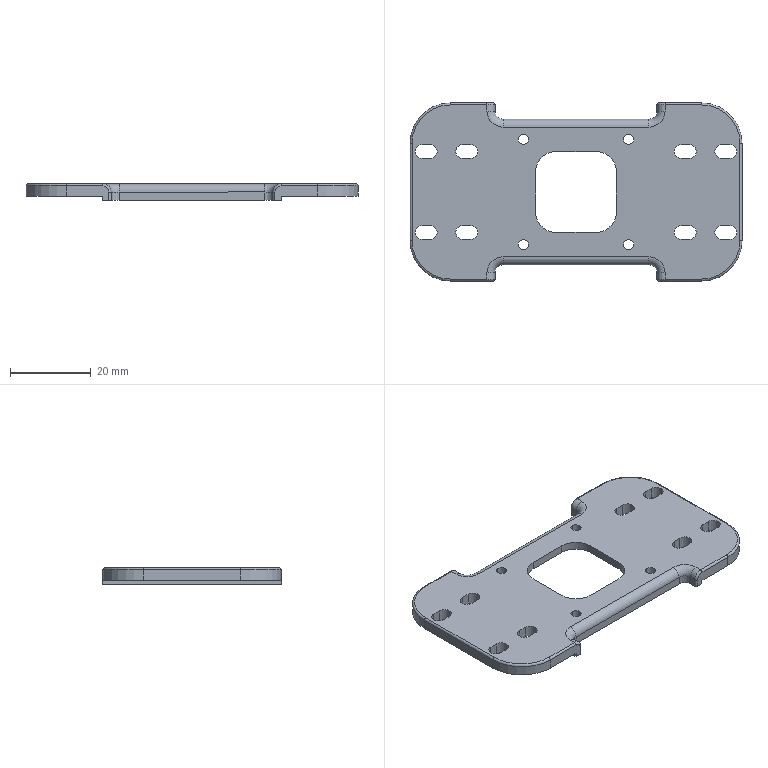NC program | NX | posted with a generic post | part box 82 x 44 x 4 mm
Lines 1 to 731 of 6362:
N10 G17 G21 G94 G90
(FLOOR_WALL , TOOL : D80)
N12 T19 M6
N14 G54
N16 G17 G0 G90 X-86. Y0. S5000 M3
N18 G43 Z30. H19
N20 Z3.
N22 G94 G1 Z0. F1200.
N24 X-83.
N26 X83.
N28 X86.
N30 Z3.
N32 G0 Z30.
N34 M5
(ZLEVEL_PROFILE , TOOL : D10)
N36 T15 M6
N38 G54
N40 G17 G0 G90 X-11.965 Y-22.757 S9500 M3
N42 G43 Z30. H15
N44 Z1.5
N46 G94 G1 X-15.396 Z1.32 F1000.
N48 X-15.532 Y-23.322 Z1.29
N50 X-16.248 Y-24.71 Z1.208
N52 X-17.318 Y-25.848 Z1.126
N54 X-18.658 Y-26.649 Z1.044
N56 X-19.213 Y-26.819 Z1.014
N58 X-19.812 Y-27.001 Z0.981
N60 X-20.411 Y-27.093 Z0.949
N62 X-21.037 Y-27.1 Z0.916
N64 X-31. Z0.394
N66 X-31.952 Z0.344
N68 X-34.354 Y-26.754 Z0.217
N70 X-36.669 Y-26.028 Z0.09
N72 X-38.838 Y-24.941 Z-0.037
N74 X-40.806 Y-23.522 Z-0.164
N76 X-42.522 Y-21.806 Z-0.291
N78 X-43.941 Y-19.838 Z-0.419
N80 X-45.028 Y-17.669 Z-0.546
N82 X-45.754 Y-15.354 Z-0.673
N84 X-46.1 Y-12.952 Z-0.8
N86 Y-12. Z-0.85
N88 Y12. F3500.
N90 G2 X-31. Y27.1 R15.1
N92 G1 X-21.037
N94 G2 X-16.327 Y24.777 R5.845
N96 X-15.396 Y22.757 R5.216
N98 G1 X15.396
N100 G2 X19.213 Y26.819 R5.615
N102 X21.037 Y27.1 R6.515
N104 G1 X31.
N106 G2 X46.1 Y12. R15.1
N108 G1 Y-12.
N110 G2 X31. Y-27.1 R15.1
N112 G1 X21.037
N114 G2 X16.327 Y-24.777 R5.845
N116 X15.396 Y-22.757 R5.216
N118 G1 X-15.396
N120 G2 X-19.213 Y-26.819 R5.615
N122 X-21.037 Y-27.1 R6.515
N124 G1 X-31.
N126 G2 X-46.1 Y-12. R15.1
N128 G1 Y12. Z-0.924
N130 X-46.072 Y12.912 Z-0.927
N132 X-45.99 Y13.82 Z-0.93
N134 X-45.853 Y14.722 Z-0.933
N136 X-45.661 Y15.614 Z-0.936
N138 X-45.416 Y16.492 Z-0.938
N140 X-45.119 Y17.355 Z-0.941
N142 X-44.77 Y18.197 Z-0.944
N144 X-44.37 Y19.017 Z-0.947
N146 X-43.922 Y19.812 Z-0.95
N148 X-43.427 Y20.578 Z-0.953
N150 X-42.886 Y21.312 Z-0.955
N152 X-42.303 Y22.013 Z-0.958
N154 X-41.677 Y22.677 Z-0.961
N156 X-41.013 Y23.303 Z-0.964
N158 X-40.312 Y23.886 Z-0.967
N160 X-39.578 Y24.427 Z-0.97
N162 X-38.812 Y24.922 Z-0.972
N164 X-38.017 Y25.37 Z-0.975
N166 X-37.197 Y25.77 Z-0.978
N168 X-36.355 Y26.119 Z-0.981
N170 X-35.492 Y26.416 Z-0.984
N172 X-34.614 Y26.661 Z-0.986
N174 X-33.722 Y26.853 Z-0.989
N176 X-32.82 Y26.99 Z-0.992
N178 X-31.912 Y27.072 Z-0.995
N180 X-31. Y27.1 Z-0.998
N182 X-21.037 Z-1.029
N184 X-20.783
N186 X-20.529 Y27.08 Z-1.03
N188 X-20.24 Y27.059 Z-1.031
N190 X-19.951 Y27.029 Z-1.032
N192 X-19.416 Y26.917 Z-1.034
N194 X-18.891 Y26.761 Z-1.035
N196 X-18.383 Y26.553 Z-1.037
N198 X-17.895 Y26.297 Z-1.039
N200 X-17.437 Y25.991 Z-1.04
N202 X-17.006 Y25.645 Z-1.042
N204 X-16.614 Y25.255 Z-1.044
N206 X-16.255 Y24.833 Z-1.046
N208 X-16.038 Y24.522 Z-1.047
N210 X-15.841 Y24.197 Z-1.048
N212 X-15.664 Y23.861 Z-1.049
N214 X-15.516 Y23.51 Z-1.05
N216 X-15.407 Y23.198 Z-1.051
N218 X-15.306 Y22.879 Z-1.052
N220 X-11.503 Y22.88 Z-1.064
N222 X-7.698 Y22.886 Z-1.076
N224 X-3.849 Y22.892 Z-1.088
N226 X0. Y22.897 Z-1.1
N228 X3.849 Y22.903 Z-1.112
N230 X7.698 Y22.908 Z-1.124
N232 X11.487 Y22.914 Z-1.136
N234 X15.276 Y22.92 Z-1.147
N236 X15.407 Y23.34 Z-1.149
N238 X15.561 Y23.743 Z-1.15
N240 X15.788 Y24.188 Z-1.152
N242 X16.043 Y24.617 Z-1.153
N244 X16.343 Y25.015 Z-1.155
N246 X16.672 Y25.389 Z-1.156
N248 X17.035 Y25.728 Z-1.158
N250 X17.425 Y26.036 Z-1.159
N252 X17.84 Y26.306 Z-1.161
N254 X18.277 Y26.537 Z-1.162
N256 X18.73 Y26.73 Z-1.164
N258 X19.197 Y26.885 Z-1.165
N260 X19.652 Y26.987 Z-1.167
N262 X20.113 Y27.056 Z-1.168
N264 X20.32 Y27.081 Z-1.169
N266 X20.528 Y27.093 Z-1.17
N268 X20.781 Y27.1
N270 X21.034 Z-1.171
N272 X31. Z-1.202
N274 X31.912 Y27.072 Z-1.205
N276 X32.82 Y26.99 Z-1.208
N278 X33.722 Y26.853 Z-1.21
N280 X34.614 Y26.661 Z-1.213
N282 X35.492 Y26.416 Z-1.216
N284 X36.355 Y26.119 Z-1.219
N286 X37.197 Y25.77 Z-1.222
N288 X38.017 Y25.37 Z-1.225
N290 X38.812 Y24.922 Z-1.227
N292 X39.578 Y24.427 Z-1.23
N294 X40.312 Y23.886 Z-1.233
N296 X41.013 Y23.303 Z-1.236
N298 X41.677 Y22.677 Z-1.239
N300 X42.303 Y22.013 Z-1.241
N302 X42.886 Y21.312 Z-1.244
N304 X43.427 Y20.578 Z-1.247
N306 X43.922 Y19.812 Z-1.25
N308 X44.37 Y19.017 Z-1.253
N310 X44.77 Y18.197 Z-1.256
N312 X45.119 Y17.355 Z-1.258
N314 X45.416 Y16.492 Z-1.261
N316 X45.661 Y15.614 Z-1.264
N318 X45.853 Y14.722 Z-1.267
N320 X45.99 Y13.82 Z-1.27
N322 X46.072 Y12.912 Z-1.273
N324 X46.1 Y12. Z-1.275
N326 Y-12. Z-1.35
N328 X46.072 Y-12.912 Z-1.353
N330 X45.99 Y-13.82 Z-1.355
N332 X45.853 Y-14.722 Z-1.358
N334 X45.661 Y-15.614 Z-1.361
N336 X45.416 Y-16.492 Z-1.364
N338 X45.119 Y-17.355 Z-1.367
N340 X44.77 Y-18.197 Z-1.369
N342 X44.37 Y-19.017 Z-1.372
N344 X43.922 Y-19.812 Z-1.375
N346 X43.427 Y-20.578 Z-1.378
N348 X42.886 Y-21.312 Z-1.381
N350 X42.303 Y-22.013 Z-1.384
N352 X41.677 Y-22.677 Z-1.386
N354 X41.013 Y-23.303 Z-1.389
N356 X40.312 Y-23.886 Z-1.392
N358 X39.578 Y-24.427 Z-1.395
N360 X38.812 Y-24.922 Z-1.398
N362 X38.017 Y-25.37 Z-1.401
N364 X37.197 Y-25.77 Z-1.403
N366 X36.355 Y-26.119 Z-1.406
N368 X35.492 Y-26.416 Z-1.409
N370 X34.614 Y-26.661 Z-1.412
N372 X33.722 Y-26.853 Z-1.415
N374 X32.82 Y-26.99 Z-1.417
N376 X31.912 Y-27.072 Z-1.42
N378 X31. Y-27.1 Z-1.423
N380 X21.037 Z-1.454
N382 X20.528 Z-1.456
N384 X20.238 Y-27.074
N386 X19.949 Y-27.045 Z-1.457
N388 X19.406 Y-26.958 Z-1.459
N390 X18.874 Y-26.815 Z-1.461
N392 X18.351 Y-26.623 Z-1.462
N394 X17.852 Y-26.376 Z-1.464
N396 X17.373 Y-26.081 Z-1.466
N398 X16.928 Y-25.737 Z-1.468
N400 X16.714 Y-25.549
N402 X16.514 Y-25.35 Z-1.469
N404 X16.324 Y-25.14 Z-1.47
N406 X16.145 Y-24.92 Z-1.471
N408 X15.917 Y-24.604 Z-1.472
N410 X15.711 Y-24.272 Z-1.474
N412 X15.529 Y-23.926 Z-1.475
N414 X15.369 Y-23.57 Z-1.476
N416 X15.277 Y-23.305 Z-1.477
N418 X15.188 Y-23.038 Z-1.478
N420 X11.444 Y-23.037 Z-1.489
N422 X7.698 Y-23.04 Z-1.501
N424 X3.849 Y-23.043 Z-1.513
N426 X0. Y-23.046 Z-1.525
N428 X-3.849 Y-23.048 Z-1.537
N430 X-7.698 Y-23.051 Z-1.549
N432 X-11.437 Y-23.053 Z-1.56
N434 X-15.176 Y-23.055 Z-1.572
N436 X-15.295 Y-23.439 Z-1.573
N438 X-15.451 Y-23.793 Z-1.574
N440 X-15.679 Y-24.25 Z-1.576
N442 X-15.953 Y-24.68 Z-1.578
N444 X-16.1 Y-24.888
N446 X-16.255 Y-25.089 Z-1.579
N448 X-16.426 Y-25.277 Z-1.58
N450 X-16.604 Y-25.458 Z-1.581
N452 X-16.977 Y-25.798 Z-1.582
N454 X-17.38 Y-26.101 Z-1.584
N456 X-17.589 Y-26.24 Z-1.585
N458 X-17.8 Y-26.375
N460 X-18.026 Y-26.483 Z-1.586
N462 X-18.252 Y-26.591 Z-1.587
N464 X-18.714 Y-26.775 Z-1.588
N466 X-19.188 Y-26.919 Z-1.59
N468 X-19.647 Y-27.017 Z-1.591
N470 X-20.111 Y-27.073 Z-1.593
N472 X-20.319 Y-27.092 Z-1.594
N474 X-20.528 Y-27.099
N476 X-20.781 Y-27.1 Z-1.595
N478 X-21.034 Z-1.596
N480 X-31. Z-1.627
N482 X-31.912 Y-27.072 Z-1.629
N484 X-32.82 Y-26.99 Z-1.632
N486 X-33.722 Y-26.853 Z-1.635
N488 X-34.614 Y-26.661 Z-1.638
N490 X-35.492 Y-26.416 Z-1.641
N492 X-36.355 Y-26.119 Z-1.644
N494 X-37.197 Y-25.77 Z-1.646
N496 X-38.017 Y-25.37 Z-1.649
N498 X-38.812 Y-24.922 Z-1.652
N500 X-39.578 Y-24.427 Z-1.655
N502 X-40.312 Y-23.886 Z-1.658
N504 X-41.013 Y-23.303 Z-1.66
N506 X-41.677 Y-22.677 Z-1.663
N508 X-42.303 Y-22.013 Z-1.666
N510 X-42.886 Y-21.312 Z-1.669
N512 X-43.427 Y-20.578 Z-1.672
N514 X-43.922 Y-19.812 Z-1.675
N516 X-44.37 Y-19.017 Z-1.677
N518 X-44.77 Y-18.197 Z-1.68
N520 X-45.119 Y-17.355 Z-1.683
N522 X-45.416 Y-16.492 Z-1.686
N524 X-45.661 Y-15.614 Z-1.689
N526 X-45.853 Y-14.722 Z-1.692
N528 X-45.99 Y-13.82 Z-1.694
N530 X-46.072 Y-12.912 Z-1.697
N532 X-46.1 Y-12. Z-1.7
N534 Y12. Z-1.774
N536 X-46.072 Y12.912 Z-1.777
N538 X-45.99 Y13.82 Z-1.78
N540 X-45.853 Y14.722 Z-1.783
N542 X-45.661 Y15.614 Z-1.786
N544 X-45.416 Y16.492 Z-1.789
N546 X-45.119 Y17.355 Z-1.791
N548 X-44.77 Y18.197 Z-1.794
N550 X-44.37 Y19.017 Z-1.797
N552 X-43.922 Y19.812 Z-1.8
N554 X-43.427 Y20.578 Z-1.803
N556 X-42.886 Y21.312 Z-1.806
N558 X-42.303 Y22.013 Z-1.808
N560 X-41.677 Y22.677 Z-1.811
N562 X-41.013 Y23.303 Z-1.814
N564 X-40.312 Y23.886 Z-1.817
N566 X-39.578 Y24.427 Z-1.82
N568 X-38.812 Y24.922 Z-1.823
N570 X-38.017 Y25.37 Z-1.825
N572 X-37.197 Y25.77 Z-1.828
N574 X-36.355 Y26.119 Z-1.831
N576 X-35.492 Y26.416 Z-1.834
N578 X-34.614 Y26.661 Z-1.837
N580 X-33.722 Y26.853 Z-1.839
N582 X-32.82 Y26.99 Z-1.842
N584 X-31.912 Y27.072 Z-1.845
N586 X-31. Y27.1 Z-1.848
N588 X-23.132 Z-1.872
N590 X-20.5 Y27.099 Z-1.881
N592 X-20.001 Y27.075 Z-1.882
N594 X-19.506 Y27.009 Z-1.884
N596 X-19.005 Y26.893 Z-1.885
N598 X-18.517 Y26.732 Z-1.887
N600 X-18.046 Y26.525 Z-1.888
N602 X-17.595 Y26.278 Z-1.89
N604 X-17.166 Y25.994 Z-1.892
N606 X-16.769 Y25.665 Z-1.893
N608 X-16.402 Y25.304 Z-1.895
N610 X-16.071 Y24.909 Z-1.896
N612 X-15.775 Y24.488 Z-1.898
N614 X-15.521 Y24.04 Z-1.9
N616 X-15.311 Y23.58 Z-1.901
N618 X-15.136 Y23.098 Z-1.903
N620 X-11.358 Z-1.914
N622 X-7.579 Y23.099 Z-1.926
N624 X-3.79 Z-1.938
N626 X0. Z-1.95
N628 X3.79 Y23.1 Z-1.961
N630 X7.579 Z-1.973
N632 X11.357 Z-1.985
N634 X15.135 Y23.099 Z-1.997
N636 X15.305 Y23.584 Z-1.998
N638 X15.513 Y24.044 Z-2.
N640 X15.767 Y24.493 Z-2.001
N642 X16.063 Y24.916 Z-2.003
N644 X16.396 Y25.31 Z-2.005
N646 X16.764 Y25.671 Z-2.006
N648 X17.163 Y25.997 Z-2.008
N650 X17.591 Y26.285 Z-2.009
N652 X18.043 Y26.532 Z-2.011
N654 X18.515 Y26.736 Z-2.013
N656 X19.004 Y26.896 Z-2.014
N658 X19.505 Y27.011 Z-2.016
N660 X20.001 Y27.078 Z-2.017
N662 X20.5 Y27.1 Z-2.019
N664 X31. Z-2.051
N666 X31.912 Y27.072 Z-2.054
N668 X32.82 Y26.99 Z-2.057
N670 X33.722 Y26.853 Z-2.06
N672 X34.614 Y26.661 Z-2.063
N674 X35.492 Y26.416 Z-2.066
N676 X36.355 Y26.119 Z-2.068
N678 X37.197 Y25.77 Z-2.071
N680 X38.017 Y25.37 Z-2.074
N682 X38.812 Y24.922 Z-2.077
N684 X39.578 Y24.427 Z-2.08
N686 X40.312 Y23.886 Z-2.083
N688 X41.013 Y23.303 Z-2.085
N690 X41.677 Y22.677 Z-2.088
N692 X42.303 Y22.013 Z-2.091
N694 X42.886 Y21.312 Z-2.094
N696 X43.427 Y20.578 Z-2.097
N698 X43.922 Y19.812 Z-2.1
N700 X44.37 Y19.017 Z-2.102
N702 X44.77 Y18.197 Z-2.105
N704 X45.119 Y17.355 Z-2.108
N706 X45.416 Y16.492 Z-2.111
N708 X45.661 Y15.614 Z-2.114
N710 X45.853 Y14.722 Z-2.117
N712 X45.99 Y13.82 Z-2.119
N714 X46.072 Y12.912 Z-2.122
N716 X46.1 Y12. Z-2.125
N718 Y-12. Z-2.199
N720 X46.072 Y-12.912 Z-2.202
N722 X45.99 Y-13.82 Z-2.205
N724 X45.853 Y-14.722 Z-2.208
N726 X45.661 Y-15.614 Z-2.211
N728 X45.416 Y-16.492 Z-2.214
N730 X45.119 Y-17.355 Z-2.216
N732 X44.77 Y-18.197 Z-2.219
N734 X44.37 Y-19.017 Z-2.222
N736 X43.922 Y-19.812 Z-2.225
N738 X43.427 Y-20.578 Z-2.228
N740 X42.886 Y-21.312 Z-2.231
N742 X42.303 Y-22.013 Z-2.233
N744 X41.677 Y-22.677 Z-2.236
N746 X41.013 Y-23.303 Z-2.239
N748 X40.312 Y-23.886 Z-2.242
N750 X39.578 Y-24.427 Z-2.245
N752 X38.812 Y-24.922 Z-2.248
N754 X38.017 Y-25.37 Z-2.25
N756 X37.197 Y-25.77 Z-2.253
N758 X36.355 Y-26.119 Z-2.256
N760 X35.492 Y-26.416 Z-2.259
N762 X34.614 Y-26.661 Z-2.262
N764 X33.722 Y-26.853 Z-2.265
N766 X32.82 Y-26.99 Z-2.267
N768 X31.912 Y-27.072 Z-2.27
N770 X31. Y-27.1 Z-2.273
N772 X20.5 Z-2.306
N774 X20.001 Y-27.078 Z-2.307
N776 X19.505 Y-27.011 Z-2.309
N778 X19.004 Y-26.896 Z-2.31
N780 X18.515 Y-26.736 Z-2.312
N782 X18.043 Y-26.532 Z-2.313
N784 X17.591 Y-26.285 Z-2.315
N786 X17.163 Y-25.997 Z-2.317
N788 X16.764 Y-25.671 Z-2.318
N790 X16.396 Y-25.31 Z-2.32
N792 X16.063 Y-24.916 Z-2.321
N794 X15.767 Y-24.493 Z-2.323
N796 X15.512 Y-24.045 Z-2.325
N798 X15.303 Y-23.585 Z-2.326
N800 X15.133 Y-23.1 Z-2.328
N802 X7.579 Z-2.351
N804 X-7.579 Z-2.398
N806 X-15.134 Z-2.422
N808 X-15.303 Y-23.586 Z-2.423
N810 X-15.512 Y-24.045 Z-2.425
N812 X-15.767 Y-24.493 Z-2.426
N814 X-16.063 Y-24.916 Z-2.428
N816 X-16.396 Y-25.31 Z-2.43
N818 X-16.764 Y-25.671 Z-2.431
N820 X-17.163 Y-25.997 Z-2.433
N822 X-17.591 Y-26.285 Z-2.434
N824 X-18.043 Y-26.532 Z-2.436
N826 X-18.515 Y-26.736 Z-2.438
N828 X-19.004 Y-26.896 Z-2.439
N830 X-19.505 Y-27.011 Z-2.441
N832 X-20.001 Y-27.078 Z-2.442
N834 X-20.5 Y-27.1 Z-2.444
N836 X-31. Z-2.476
N838 X-31.912 Y-27.072 Z-2.479
N840 X-32.82 Y-26.99 Z-2.482
N842 X-33.722 Y-26.853 Z-2.485
N844 X-34.614 Y-26.661 Z-2.488
N846 X-35.492 Y-26.416 Z-2.491
N848 X-36.355 Y-26.119 Z-2.493
N850 X-37.197 Y-25.77 Z-2.496
N852 X-38.017 Y-25.37 Z-2.499
N854 X-38.812 Y-24.922 Z-2.502
N856 X-39.578 Y-24.427 Z-2.505
N858 X-40.312 Y-23.886 Z-2.508
N860 X-41.013 Y-23.303 Z-2.51
N862 X-41.677 Y-22.677 Z-2.513
N864 X-42.303 Y-22.013 Z-2.516
N866 X-42.886 Y-21.312 Z-2.519
N868 X-43.427 Y-20.578 Z-2.522
N870 X-43.922 Y-19.812 Z-2.525
N872 X-44.37 Y-19.017 Z-2.527
N874 X-44.77 Y-18.197 Z-2.53
N876 X-45.119 Y-17.355 Z-2.533
N878 X-45.416 Y-16.492 Z-2.536
N880 X-45.661 Y-15.614 Z-2.539
N882 X-45.853 Y-14.722 Z-2.542
N884 X-45.99 Y-13.82 Z-2.544
N886 X-46.072 Y-12.912 Z-2.547
N888 X-46.1 Y-12. Z-2.55
N890 Y12. Z-2.624
N892 X-46.072 Y12.912 Z-2.627
N894 X-45.99 Y13.82 Z-2.63
N896 X-45.853 Y14.722 Z-2.633
N898 X-45.661 Y15.614 Z-2.636
N900 X-45.416 Y16.492 Z-2.639
N902 X-45.119 Y17.355 Z-2.641
N904 X-44.77 Y18.197 Z-2.644
N906 X-44.37 Y19.017 Z-2.647
N908 X-43.922 Y19.812 Z-2.65
N910 X-43.427 Y20.578 Z-2.653
N912 X-42.886 Y21.312 Z-2.656
N914 X-42.303 Y22.013 Z-2.658
N916 X-41.677 Y22.677 Z-2.661
N918 X-41.013 Y23.303 Z-2.664
N920 X-40.312 Y23.886 Z-2.667
N922 X-39.578 Y24.427 Z-2.67
N924 X-38.812 Y24.922 Z-2.673
N926 X-38.017 Y25.37 Z-2.675
N928 X-37.197 Y25.77 Z-2.678
N930 X-36.355 Y26.119 Z-2.681
N932 X-35.492 Y26.416 Z-2.684
N934 X-34.614 Y26.661 Z-2.687
N936 X-33.722 Y26.853 Z-2.69
N938 X-32.82 Y26.99 Z-2.692
N940 X-31.912 Y27.072 Z-2.695
N942 X-31. Y27.1 Z-2.698
N944 X-20.5 Z-2.731
N946 X-19.988 Y27.077 Z-2.732
N948 X-19.481 Y27.006 Z-2.734
N950 X-18.982 Y26.89 Z-2.735
N952 X-18.496 Y26.729 Z-2.737
N954 X-18.026 Y26.524 Z-2.738
N956 X-17.578 Y26.277 Z-2.74
N958 X-17.153 Y25.99 Z-2.742
N960 X-16.757 Y25.665 Z-2.743
N962 X-16.392 Y25.306 Z-2.745
N964 X-16.062 Y24.915 Z-2.746
N966 X-15.768 Y24.495 Z-2.748
N968 X-15.514 Y24.05 Z-2.75
N970 X-15.305 Y23.591 Z-2.751
N972 X-15.133 Y23.1 Z-2.753
N974 X-11.35 Z-2.765
N976 X7.567 Z-2.823
N978 X11.35 Z-2.835
N980 X15.133 Z-2.847
N982 X15.305 Y23.591 Z-2.848
N984 X15.514 Y24.05 Z-2.85
N986 X15.768 Y24.495 Z-2.851
N988 X16.062 Y24.915 Z-2.853
N990 X16.392 Y25.306 Z-2.855
N992 X16.757 Y25.665 Z-2.856
N994 X17.153 Y25.99 Z-2.858
N996 X17.578 Y26.277 Z-2.859
N998 X18.026 Y26.524 Z-2.861
N1000 X18.496 Y26.729 Z-2.863
N1002 X18.982 Y26.89 Z-2.864
N1004 X19.481 Y27.006 Z-2.866
N1006 X19.988 Y27.077 Z-2.867
N1008 X20.5 Y27.1 Z-2.869
N1010 X31. Z-2.901
N1012 X31.912 Y27.072 Z-2.904
N1014 X32.82 Y26.99 Z-2.907
N1016 X33.722 Y26.853 Z-2.91
N1018 X34.614 Y26.661 Z-2.913
N1020 X35.492 Y26.416 Z-2.916
N1022 X36.355 Y26.119 Z-2.918
N1024 X37.197 Y25.77 Z-2.921
N1026 X38.017 Y25.37 Z-2.924
N1028 X38.812 Y24.922 Z-2.927
N1030 X39.578 Y24.427 Z-2.93
N1032 X40.312 Y23.886 Z-2.933
N1034 X41.013 Y23.303 Z-2.935
N1036 X41.677 Y22.677 Z-2.938
N1038 X42.303 Y22.013 Z-2.941
N1040 X42.886 Y21.312 Z-2.944
N1042 X43.427 Y20.578 Z-2.947
N1044 X43.922 Y19.812 Z-2.95
N1046 X44.37 Y19.017 Z-2.952
N1048 X44.77 Y18.197 Z-2.955
N1050 X45.119 Y17.355 Z-2.958
N1052 X45.416 Y16.492 Z-2.961
N1054 X45.661 Y15.614 Z-2.964
N1056 X45.853 Y14.722 Z-2.967
N1058 X45.99 Y13.82 Z-2.969
N1060 X46.072 Y12.912 Z-2.972
N1062 X46.1 Y12. Z-2.975
N1064 Y-12. Z-3.049
N1066 X46.072 Y-12.912 Z-3.052
N1068 X45.99 Y-13.82 Z-3.055
N1070 X45.853 Y-14.722 Z-3.058
N1072 X45.661 Y-15.614 Z-3.061
N1074 X45.416 Y-16.492 Z-3.064
N1076 X45.119 Y-17.355 Z-3.066
N1078 X44.77 Y-18.197 Z-3.069
N1080 X44.37 Y-19.017 Z-3.072
N1082 X43.922 Y-19.812 Z-3.075
N1084 X43.427 Y-20.578 Z-3.078
N1086 X42.886 Y-21.312 Z-3.081
N1088 X42.303 Y-22.013 Z-3.083
N1090 X41.677 Y-22.677 Z-3.086
N1092 X41.013 Y-23.303 Z-3.089
N1094 X40.312 Y-23.886 Z-3.092
N1096 X39.578 Y-24.427 Z-3.095
N1098 X38.812 Y-24.922 Z-3.098
N1100 X38.017 Y-25.37 Z-3.1
N1102 X37.197 Y-25.77 Z-3.103
N1104 X36.355 Y-26.119 Z-3.106
N1106 X35.492 Y-26.416 Z-3.109
N1108 X34.614 Y-26.661 Z-3.112
N1110 X33.722 Y-26.853 Z-3.115
N1112 X32.82 Y-26.99 Z-3.117
N1114 X31.912 Y-27.072 Z-3.12
N1116 X31. Y-27.1 Z-3.123
N1118 X20.5 Z-3.156
N1120 X19.988 Y-27.077 Z-3.157
N1122 X19.481 Y-27.006 Z-3.159
N1124 X18.982 Y-26.89 Z-3.16
N1126 X18.496 Y-26.729 Z-3.162
N1128 X18.026 Y-26.524 Z-3.163
N1130 X17.578 Y-26.277 Z-3.165
N1132 X17.153 Y-25.99 Z-3.167
N1134 X16.757 Y-25.665 Z-3.168
N1136 X16.392 Y-25.306 Z-3.17
N1138 X16.062 Y-24.915 Z-3.171
N1140 X15.768 Y-24.495 Z-3.173
N1142 X15.514 Y-24.05 Z-3.175
N1144 X15.305 Y-23.591 Z-3.176
N1146 X15.133 Y-23.1 Z-3.178
N1148 X-15.134 Z-3.272
N1150 X-15.305 Y-23.591 Z-3.273
N1152 X-15.514 Y-24.05 Z-3.275
N1154 X-15.768 Y-24.495 Z-3.276
N1156 X-16.062 Y-24.915 Z-3.278
N1158 X-16.392 Y-25.306 Z-3.28
N1160 X-16.757 Y-25.665 Z-3.281
N1162 X-17.153 Y-25.99 Z-3.283
N1164 X-17.578 Y-26.277 Z-3.284
N1166 X-18.026 Y-26.524 Z-3.286
N1168 X-18.496 Y-26.729 Z-3.288
N1170 X-18.982 Y-26.89 Z-3.289
N1172 X-19.481 Y-27.006 Z-3.291
N1174 X-19.988 Y-27.077 Z-3.292
N1176 X-20.5 Y-27.1 Z-3.294
N1178 X-31. Z-3.326
N1180 X-31.912 Y-27.072 Z-3.329
N1182 X-32.82 Y-26.99 Z-3.332
N1184 X-33.722 Y-26.853 Z-3.335
N1186 X-34.614 Y-26.661 Z-3.338
N1188 X-35.492 Y-26.416 Z-3.341
N1190 X-36.355 Y-26.119 Z-3.343
N1192 X-37.197 Y-25.77 Z-3.346
N1194 X-38.017 Y-25.37 Z-3.349
N1196 X-38.812 Y-24.922 Z-3.352
N1198 X-39.578 Y-24.427 Z-3.355
N1200 X-40.312 Y-23.886 Z-3.358
N1202 X-41.013 Y-23.303 Z-3.36
N1204 X-41.677 Y-22.677 Z-3.363
N1206 X-42.303 Y-22.013 Z-3.366
N1208 X-42.886 Y-21.312 Z-3.369
N1210 X-43.427 Y-20.578 Z-3.372
N1212 X-43.922 Y-19.812 Z-3.375
N1214 X-44.37 Y-19.017 Z-3.377
N1216 X-44.77 Y-18.197 Z-3.38
N1218 X-45.119 Y-17.355 Z-3.383
N1220 X-45.416 Y-16.492 Z-3.386
N1222 X-45.661 Y-15.614 Z-3.389
N1224 X-45.853 Y-14.722 Z-3.392
N1226 X-45.99 Y-13.82 Z-3.394
N1228 X-46.072 Y-12.912 Z-3.397
N1230 X-46.1 Y-12. Z-3.4
N1232 Y12.
N1234 G2 X-31. Y27.1 R15.1
N1236 G1 X-20.5
N1238 G2 X-15.133 Y23.1 R5.6
N1240 G1 X15.133
N1242 G2 X20.5 Y27.1 R5.6
N1244 G1 X31.
N1246 G2 X46.1 Y12. R15.1
N1248 G1 Y-12.
N1250 G2 X31. Y-27.1 R15.1
N1252 G1 X20.5
N1254 G2 X15.133 Y-23.1 R5.6
N1256 G1 X-15.134
N1258 G2 X-20.5 Y-27.1 R5.6
N1260 G1 X-31.
N1262 G2 X-46.1 Y-12. R15.1
N1264 G1 Z-1.9
N1266 G0 Z30.
(PLANAR_MILL_3 , TOOL : D10)
N1268 X-4.9 Y-1.297
N1270 Z1.5
N1272 G1 Y-4.9 Z1.311 F1000.
N1274 X4.9 Z0.798
N1276 Y4.9 Z0.284
N1278 X-4.9 Z-0.23
N1280 Y-4.9 Z-0.743
N1282 X0. Z-1.
N1284 Y-0.4
N1286 X0.4 F3500.
N1288 Y0.4
N1290 X-0.4
N1292 Y-0.4
N1294 X0.
N1296 Y-4.9
N1298 X4.9
N1300 Y4.9
N1302 X-4.9
N1304 Y-4.9
N1306 X0.
N1308 Z0.5
N1310 G0 X-4.9 Y-1.297
N1312 G1 Y-4.9 Z0.311 F1000.
N1314 X4.9 Z-0.202
N1316 Y4.9 Z-0.716
N1318 X-4.9 Z-1.23
N1320 Y-4.9 Z-1.743
N1322 X0. Z-2.
N1324 Y-0.4
N1326 X0.4 F3500.
N1328 Y0.4
N1330 X-0.4
N1332 Y-0.4
N1334 X0.
N1336 Y-4.9
N1338 X4.9
N1340 Y4.9
N1342 X-4.9
N1344 Y-4.9
N1346 X0.
N1348 Z-0.5
N1350 G0 Z30.
N1352 M5
(ZLEVEL_PROFILE_COPY_COPY , TOOL : D10JING)
N1354 T14 M6
N1356 G54
N1358 G17 G0 G90 X2.536 Y3. S9500 M3
N1360 G43 Z30. H14
N1362 Z-1.
N1364 G94 G1 Z-2. F1000.
N1366 X4.5 Y4.134
N1368 G3 X5. Y5. R1.
N1370 G1 X-5. F1500.
N1372 Y-5.
N1374 X5.
N1376 Y5.
N1378 G3 X4.134 Y4.5 R1.
N1380 G1 X3. Y2.536
N1382 Z-1.
N1384 G0 Z30.
N1386 M5
(SPOT_DRILLING , TOOL : D6A45)
N1388 T01 M6
N1390 G54
N1392 G17 G0 G90 X13. Y13. S9500 M3
N1394 G43 Z30. H1
N1396 G94 G82 G98 Z-1. F250. P200 R3.
N1398 X-13.
N1400 Y-13.
N1402 X13.
N1404 G80
N1406 G0 X13. Y-13. Z30.
N1408 M5
(SPOT_DRILLING_COPY , TOOL : 2.5ZT)
N1410 T02 M6
N1412 G54
N1414 G17 G0 G90 X13. Y13. S2500 M3
N1416 G43 Z30. H2
N1418 G94 G83 G98 Z-4.751 F120. Q2. R3.
N1420 X-13.
N1422 Y-13.
N1424 X13.
N1426 G80
N1428 G0 X13. Y-13. Z30.
N1430 M5